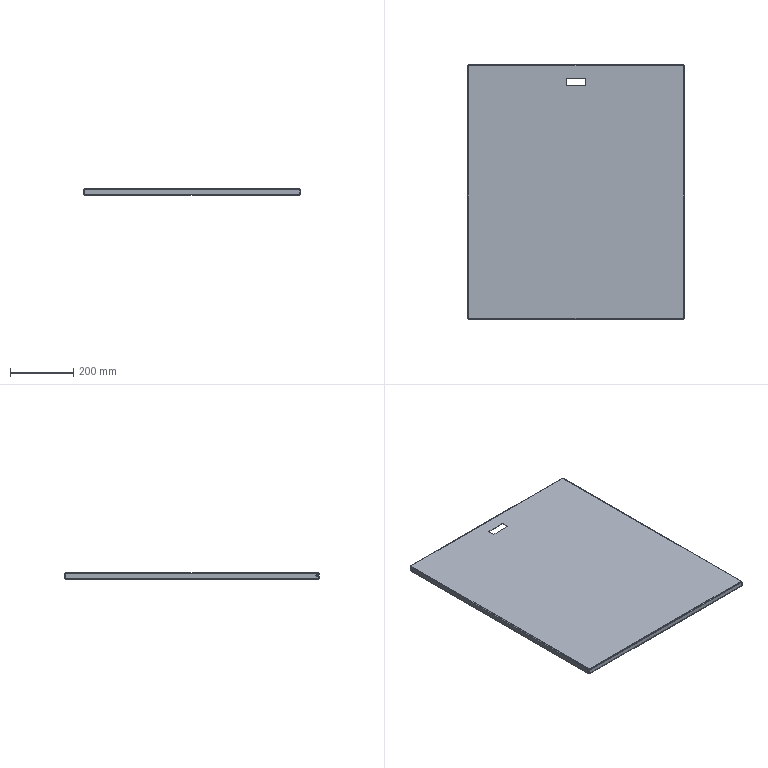Part | STEP file | Rear door panel V1.201001 | 1 solid | 78 faces | box 686 x 805 x 19 mm | volume 939207 mm3 | plane 42 | cylinder 20 | spline 16 | commonest cylinder face diameters 3 x8 6 x8 5 x4